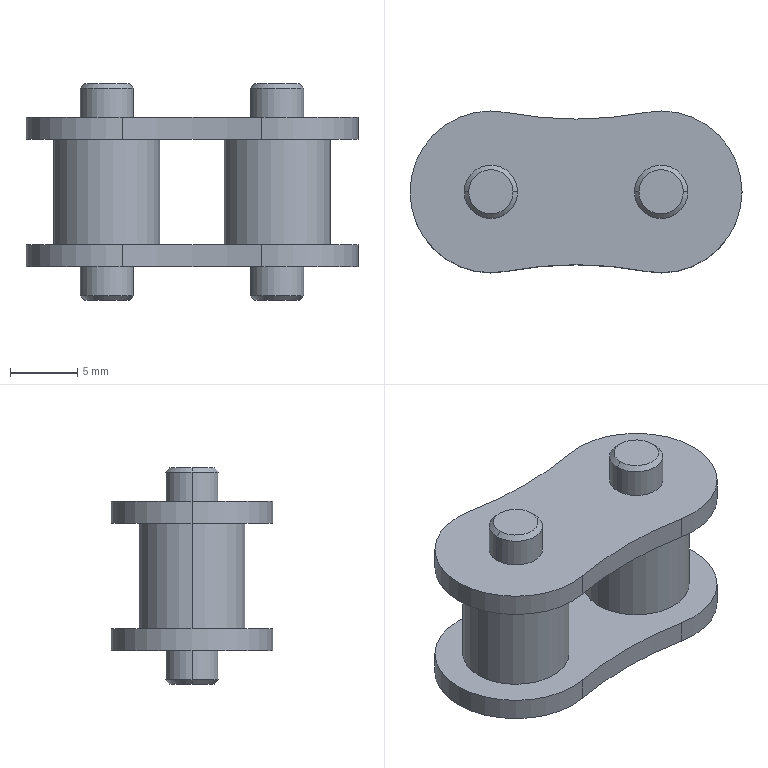Part | SolidWorks | features Boss 2, Chamfer 1, Extrusion 1, MirrorPattern 1 | 1 solid | 38 faces | box 24.77 x 12.07 x 16.175 mm | volume 1756 mm3 | cylinder 22 | cone 8 | plane 8 | commonest cylinder face diameters 3.98 x8 12.07 x6 7.92 x4 55.348 x4
STEP:
#1=CARTESIAN_POINT('',(-8.007,0.,-8.087));
#2=VERTEX_POINT('',#1);
#3=CARTESIAN_POINT('',(-4.693,0.,-8.087));
#4=VERTEX_POINT('',#3);
#5=CARTESIAN_POINT('',(-6.35,0.,-8.087));
#6=DIRECTION('',(0.,0.,-1.));
#7=DIRECTION('',(-1.,0.,0.));
#8=AXIS2_PLACEMENT_3D('',#5,#6,#7);
#9=CIRCLE('',#8,1.657);
#10=EDGE_CURVE('',#2,#4,#9,.T.);
#11=ORIENTED_EDGE('',*,*,#10,.F.);
#12=CARTESIAN_POINT('',(-8.34,0.,-7.754));
#13=VERTEX_POINT('',#12);
#14=CARTESIAN_POINT('',(-8.34,0.,-7.754));
#15=DIRECTION('',(-0.7071,0.,0.7071));
#16=VECTOR('',#15,1000.);
#17=LINE('',#14,#16);
#18=EDGE_CURVE('',#2,#13,#17,.T.);
#19=ORIENTED_EDGE('',*,*,#18,.T.);
#20=CARTESIAN_POINT('',(-4.36,0.,-7.754));
#21=VERTEX_POINT('',#20);
#22=CARTESIAN_POINT('',(-6.35,0.,-7.754));
#23=DIRECTION('',(0.,0.,1.));
#24=DIRECTION('',(-1.,0.,0.));
#25=AXIS2_PLACEMENT_3D('',#22,#23,#24);
#26=CIRCLE('',#25,1.99);
#27=EDGE_CURVE('',#21,#13,#26,.T.);
#28=ORIENTED_EDGE('',*,*,#27,.F.);
#29=CARTESIAN_POINT('',(-4.36,0.,-7.754));
#30=DIRECTION('',(0.7071,0.,0.7071));
#31=VECTOR('',#30,1000.);
#32=LINE('',#29,#31);
#33=EDGE_CURVE('',#4,#21,#32,.T.);
#34=ORIENTED_EDGE('',*,*,#33,.F.);
#35=EDGE_LOOP('',(#11,#19,#28,#34));
#36=FACE_OUTER_BOUND('',#35,.T.);
#37=CARTESIAN_POINT('',(-6.35,0.,-7.754));
#38=DIRECTION('',(0.,0.,1.));
#39=DIRECTION('',(1.,0.,0.));
#40=AXIS2_PLACEMENT_3D('',#37,#38,#39);
#41=CONICAL_SURFACE('',#40,1.99,0.7854);
#42=ADVANCED_FACE('',(#36),#41,.T.);
#43=CARTESIAN_POINT('',(4.693,0.,-8.087));
#44=VERTEX_POINT('',#43);
#45=CARTESIAN_POINT('',(8.007,0.,-8.087));
#46=VERTEX_POINT('',#45);
#47=CARTESIAN_POINT('',(6.35,0.,-8.087));
#48=DIRECTION('',(0.,0.,-1.));
#49=DIRECTION('',(-1.,0.,0.));
#50=AXIS2_PLACEMENT_3D('',#47,#48,#49);
#51=CIRCLE('',#50,1.657);
#52=EDGE_CURVE('',#44,#46,#51,.T.);
#53=ORIENTED_EDGE('',*,*,#52,.F.);
#54=CARTESIAN_POINT('',(4.36,0.,-7.754));
#55=VERTEX_POINT('',#54);
#56=CARTESIAN_POINT('',(4.36,0.,-7.754));
#57=DIRECTION('',(-0.7071,0.,0.7071));
#58=VECTOR('',#57,1000.);
#59=LINE('',#56,#58);
#60=EDGE_CURVE('',#44,#55,#59,.T.);
#61=ORIENTED_EDGE('',*,*,#60,.T.);
#62=CARTESIAN_POINT('',(8.34,0.,-7.754));
#63=VERTEX_POINT('',#62);
#64=CARTESIAN_POINT('',(6.35,0.,-7.754));
#65=DIRECTION('',(0.,0.,1.));
#66=DIRECTION('',(-1.,0.,0.));
#67=AXIS2_PLACEMENT_3D('',#64,#65,#66);
#68=CIRCLE('',#67,1.99);
#69=EDGE_CURVE('',#63,#55,#68,.T.);
#70=ORIENTED_EDGE('',*,*,#69,.F.);
#71=CARTESIAN_POINT('',(8.34,0.,-7.754));
#72=DIRECTION('',(0.7071,0.,0.7071));
#73=VECTOR('',#72,1000.);
#74=LINE('',#71,#73);
#75=EDGE_CURVE('',#46,#63,#74,.T.);
#76=ORIENTED_EDGE('',*,*,#75,.F.);
#77=EDGE_LOOP('',(#53,#61,#70,#76));
#78=FACE_OUTER_BOUND('',#77,.T.);
#79=CARTESIAN_POINT('',(6.35,0.,-7.754));
#80=DIRECTION('',(0.,0.,1.));
#81=DIRECTION('',(1.,0.,0.));
#82=AXIS2_PLACEMENT_3D('',#79,#80,#81);
#83=CONICAL_SURFACE('',#82,1.99,0.7854);
#84=ADVANCED_FACE('',(#78),#83,.T.);
#85=ORIENTED_EDGE('',*,*,#27,.T.);
#86=CARTESIAN_POINT('',(-8.34,0.,-5.59));
#87=VERTEX_POINT('',#86);
#88=CARTESIAN_POINT('',(-8.34,0.,-8.087));
#89=DIRECTION('',(0.,0.,1.));
#90=VECTOR('',#89,1000.);
#91=LINE('',#88,#90);
#92=EDGE_CURVE('',#13,#87,#91,.T.);
#93=ORIENTED_EDGE('',*,*,#92,.T.);
#94=CARTESIAN_POINT('',(-4.36,0.,-5.59));
#95=VERTEX_POINT('',#94);
#96=CARTESIAN_POINT('',(-6.35,0.,-5.59));
#97=DIRECTION('',(0.,0.,-1.));
#98=DIRECTION('',(-1.,0.,0.));
#99=AXIS2_PLACEMENT_3D('',#96,#97,#98);
#100=CIRCLE('',#99,1.99);
#101=EDGE_CURVE('',#87,#95,#100,.T.);
#102=ORIENTED_EDGE('',*,*,#101,.T.);
#103=CARTESIAN_POINT('',(-4.36,0.,-8.087));
#104=DIRECTION('',(0.,0.,1.));
#105=VECTOR('',#104,1000.);
#106=LINE('',#103,#105);
#107=EDGE_CURVE('',#21,#95,#106,.T.);
#108=ORIENTED_EDGE('',*,*,#107,.F.);
#109=EDGE_LOOP('',(#85,#93,#102,#108));
#110=FACE_OUTER_BOUND('',#109,.T.);
#111=CARTESIAN_POINT('',(-6.35,0.,-8.087));
#112=DIRECTION('',(0.,0.,1.));
#113=DIRECTION('',(1.,0.,0.));
#114=AXIS2_PLACEMENT_3D('',#111,#112,#113);
#115=CYLINDRICAL_SURFACE('',#114,1.99);
#116=ADVANCED_FACE('',(#110),#115,.T.);
#117=ORIENTED_EDGE('',*,*,#69,.T.);
#118=CARTESIAN_POINT('',(4.36,0.,-5.59));
#119=VERTEX_POINT('',#118);
#120=CARTESIAN_POINT('',(4.36,0.,-8.087));
#121=DIRECTION('',(0.,0.,1.));
#122=VECTOR('',#121,1000.);
#123=LINE('',#120,#122);
#124=EDGE_CURVE('',#55,#119,#123,.T.);
#125=ORIENTED_EDGE('',*,*,#124,.T.);
#126=CARTESIAN_POINT('',(8.34,0.,-5.59));
#127=VERTEX_POINT('',#126);
#128=CARTESIAN_POINT('',(6.35,0.,-5.59));
#129=DIRECTION('',(0.,0.,-1.));
#130=DIRECTION('',(-1.,0.,0.));
#131=AXIS2_PLACEMENT_3D('',#128,#129,#130);
#132=CIRCLE('',#131,1.99);
#133=EDGE_CURVE('',#119,#127,#132,.T.);
#134=ORIENTED_EDGE('',*,*,#133,.T.);
#135=CARTESIAN_POINT('',(8.34,0.,-8.087));
#136=DIRECTION('',(0.,0.,1.));
#137=VECTOR('',#136,1000.);
#138=LINE('',#135,#137);
#139=EDGE_CURVE('',#63,#127,#138,.T.);
#140=ORIENTED_EDGE('',*,*,#139,.F.);
#141=EDGE_LOOP('',(#117,#125,#134,#140));
#142=FACE_OUTER_BOUND('',#141,.T.);
#143=CARTESIAN_POINT('',(6.35,0.,-8.087));
#144=DIRECTION('',(0.,0.,1.));
#145=DIRECTION('',(1.,0.,0.));
#146=AXIS2_PLACEMENT_3D('',#143,#144,#145);
#147=CYLINDRICAL_SURFACE('',#146,1.99);
#148=ADVANCED_FACE('',(#142),#147,.T.);
#149=CARTESIAN_POINT('',(5.213,-5.927,-5.59));
#150=VERTEX_POINT('',#149);
#151=CARTESIAN_POINT('',(12.385,0.,-5.59));
#152=VERTEX_POINT('',#151);
#153=CARTESIAN_POINT('',(6.35,0.,-5.59));
#154=DIRECTION('',(0.,0.,1.));
#155=DIRECTION('',(1.,0.,0.));
#156=AXIS2_PLACEMENT_3D('',#153,#154,#155);
#157=CIRCLE('',#156,6.035);
#158=EDGE_CURVE('',#150,#152,#157,.T.);
#159=ORIENTED_EDGE('',*,*,#158,.T.);
#160=CARTESIAN_POINT('',(12.385,0.,-3.925));
#161=VERTEX_POINT('',#160);
#162=CARTESIAN_POINT('',(12.385,0.,-5.59));
#163=DIRECTION('',(0.,0.,1.));
#164=VECTOR('',#163,1000.);
#165=LINE('',#162,#164);
#166=EDGE_CURVE('',#152,#161,#165,.T.);
#167=ORIENTED_EDGE('',*,*,#166,.T.);
#168=CARTESIAN_POINT('',(5.213,-5.927,-3.925));
#169=VERTEX_POINT('',#168);
#170=CARTESIAN_POINT('',(6.35,0.,-3.925));
#171=DIRECTION('',(0.,0.,1.));
#172=DIRECTION('',(1.,0.,0.));
#173=AXIS2_PLACEMENT_3D('',#170,#171,#172);
#174=CIRCLE('',#173,6.035);
#175=EDGE_CURVE('',#169,#161,#174,.T.);
#176=ORIENTED_EDGE('',*,*,#175,.F.);
#177=CARTESIAN_POINT('',(5.213,-5.927,-5.59));
#178=DIRECTION('',(0.,0.,1.));
#179=VECTOR('',#178,1000.);
#180=LINE('',#177,#179);
#181=EDGE_CURVE('',#150,#169,#180,.T.);
#182=ORIENTED_EDGE('',*,*,#181,.F.);
#183=EDGE_LOOP('',(#159,#167,#176,#182));
#184=FACE_OUTER_BOUND('',#183,.T.);
#185=CARTESIAN_POINT('',(6.35,0.,-5.59));
#186=DIRECTION('',(0.,0.,1.));
#187=DIRECTION('',(1.,0.,0.));
#188=AXIS2_PLACEMENT_3D('',#185,#186,#187);
#189=CYLINDRICAL_SURFACE('',#188,6.035);
#190=ADVANCED_FACE('',(#184),#189,.T.);
#191=CARTESIAN_POINT('',(-4.693,0.,8.087));
#192=VERTEX_POINT('',#191);
#193=CARTESIAN_POINT('',(-8.007,0.,8.087));
#194=VERTEX_POINT('',#193);
#195=CARTESIAN_POINT('',(-6.35,0.,8.087));
#196=DIRECTION('',(0.,0.,1.));
#197=DIRECTION('',(1.,0.,0.));
#198=AXIS2_PLACEMENT_3D('',#195,#196,#197);
#199=CIRCLE('',#198,1.657);
#200=EDGE_CURVE('',#192,#194,#199,.T.);
#201=ORIENTED_EDGE('',*,*,#200,.F.);
#202=CARTESIAN_POINT('',(-4.36,0.,7.754));
#203=VERTEX_POINT('',#202);
#204=CARTESIAN_POINT('',(-4.693,0.,8.087));
#205=DIRECTION('',(0.7071,0.,-0.7071));
#206=VECTOR('',#205,1000.);
#207=LINE('',#204,#206);
#208=EDGE_CURVE('',#192,#203,#207,.T.);
#209=ORIENTED_EDGE('',*,*,#208,.T.);
#210=CARTESIAN_POINT('',(-8.34,0.,7.754));
#211=VERTEX_POINT('',#210);
#212=CARTESIAN_POINT('',(-6.35,0.,7.754));
#213=DIRECTION('',(0.,0.,-1.));
#214=DIRECTION('',(1.,0.,0.));
#215=AXIS2_PLACEMENT_3D('',#212,#213,#214);
#216=CIRCLE('',#215,1.99);
#217=EDGE_CURVE('',#211,#203,#216,.T.);
#218=ORIENTED_EDGE('',*,*,#217,.F.);
#219=CARTESIAN_POINT('',(-8.007,0.,8.087));
#220=DIRECTION('',(-0.7071,0.,-0.7071));
#221=VECTOR('',#220,1000.);
#222=LINE('',#219,#221);
#223=EDGE_CURVE('',#194,#211,#222,.T.);
#224=ORIENTED_EDGE('',*,*,#223,.F.);
#225=EDGE_LOOP('',(#201,#209,#218,#224));
#226=FACE_OUTER_BOUND('',#225,.T.);
#227=CARTESIAN_POINT('',(-6.35,0.,8.087));
#228=DIRECTION('',(0.,0.,-1.));
#229=DIRECTION('',(-1.,0.,0.));
#230=AXIS2_PLACEMENT_3D('',#227,#228,#229);
#231=CONICAL_SURFACE('',#230,1.657,0.7854);
#232=ADVANCED_FACE('',(#226),#231,.T.);
#233=CARTESIAN_POINT('',(8.007,0.,8.087));
#234=VERTEX_POINT('',#233);
#235=CARTESIAN_POINT('',(4.693,0.,8.087));
#236=VERTEX_POINT('',#235);
#237=CARTESIAN_POINT('',(6.35,0.,8.087));
#238=DIRECTION('',(0.,0.,1.));
#239=DIRECTION('',(1.,0.,0.));
#240=AXIS2_PLACEMENT_3D('',#237,#238,#239);
#241=CIRCLE('',#240,1.657);
#242=EDGE_CURVE('',#234,#236,#241,.T.);
#243=ORIENTED_EDGE('',*,*,#242,.F.);
#244=CARTESIAN_POINT('',(8.34,0.,7.754));
#245=VERTEX_POINT('',#244);
#246=CARTESIAN_POINT('',(8.007,0.,8.087));
#247=DIRECTION('',(0.7071,0.,-0.7071));
#248=VECTOR('',#247,1000.);
#249=LINE('',#246,#248);
#250=EDGE_CURVE('',#234,#245,#249,.T.);
#251=ORIENTED_EDGE('',*,*,#250,.T.);
#252=CARTESIAN_POINT('',(4.36,0.,7.754));
#253=VERTEX_POINT('',#252);
#254=CARTESIAN_POINT('',(6.35,0.,7.754));
#255=DIRECTION('',(0.,0.,-1.));
#256=DIRECTION('',(1.,0.,0.));
#257=AXIS2_PLACEMENT_3D('',#254,#255,#256);
#258=CIRCLE('',#257,1.99);
#259=EDGE_CURVE('',#253,#245,#258,.T.);
#260=ORIENTED_EDGE('',*,*,#259,.F.);
#261=CARTESIAN_POINT('',(4.693,0.,8.087));
#262=DIRECTION('',(-0.7071,0.,-0.7071));
#263=VECTOR('',#262,1000.);
#264=LINE('',#261,#263);
#265=EDGE_CURVE('',#236,#253,#264,.T.);
#266=ORIENTED_EDGE('',*,*,#265,.F.);
#267=EDGE_LOOP('',(#243,#251,#260,#266));
#268=FACE_OUTER_BOUND('',#267,.T.);
#269=CARTESIAN_POINT('',(6.35,0.,8.087));
#270=DIRECTION('',(0.,0.,-1.));
#271=DIRECTION('',(-1.,0.,0.));
#272=AXIS2_PLACEMENT_3D('',#269,#270,#271);
#273=CONICAL_SURFACE('',#272,1.657,0.7854);
#274=ADVANCED_FACE('',(#268),#273,.T.);
#275=ORIENTED_EDGE('',*,*,#217,.T.);
#276=CARTESIAN_POINT('',(-4.36,0.,5.59));
#277=VERTEX_POINT('',#276);
#278=CARTESIAN_POINT('',(-4.36,0.,8.087));
#279=DIRECTION('',(0.,0.,-1.));
#280=VECTOR('',#279,1000.);
#281=LINE('',#278,#280);
#282=EDGE_CURVE('',#203,#277,#281,.T.);
#283=ORIENTED_EDGE('',*,*,#282,.T.);
#284=CARTESIAN_POINT('',(-8.34,0.,5.59));
#285=VERTEX_POINT('',#284);
#286=CARTESIAN_POINT('',(-6.35,0.,5.59));
#287=DIRECTION('',(0.,0.,1.));
#288=DIRECTION('',(1.,0.,0.));
#289=AXIS2_PLACEMENT_3D('',#286,#287,#288);
#290=CIRCLE('',#289,1.99);
#291=EDGE_CURVE('',#277,#285,#290,.T.);
#292=ORIENTED_EDGE('',*,*,#291,.T.);
#293=CARTESIAN_POINT('',(-8.34,0.,8.087));
#294=DIRECTION('',(0.,0.,-1.));
#295=VECTOR('',#294,1000.);
#296=LINE('',#293,#295);
#297=EDGE_CURVE('',#211,#285,#296,.T.);
#298=ORIENTED_EDGE('',*,*,#297,.F.);
#299=EDGE_LOOP('',(#275,#283,#292,#298));
#300=FACE_OUTER_BOUND('',#299,.T.);
#301=CARTESIAN_POINT('',(-6.35,0.,8.087));
#302=DIRECTION('',(0.,0.,-1.));
#303=DIRECTION('',(-1.,0.,0.));
#304=AXIS2_PLACEMENT_3D('',#301,#302,#303);
#305=CYLINDRICAL_SURFACE('',#304,1.99);
#306=ADVANCED_FACE('',(#300),#305,.T.);
#307=ORIENTED_EDGE('',*,*,#259,.T.);
#308=CARTESIAN_POINT('',(8.34,0.,5.59));
#309=VERTEX_POINT('',#308);
#310=CARTESIAN_POINT('',(8.34,0.,8.087));
#311=DIRECTION('',(0.,0.,-1.));
#312=VECTOR('',#311,1000.);
#313=LINE('',#310,#312);
#314=EDGE_CURVE('',#245,#309,#313,.T.);
#315=ORIENTED_EDGE('',*,*,#314,.T.);
#316=CARTESIAN_POINT('',(4.36,0.,5.59));
#317=VERTEX_POINT('',#316);
#318=CARTESIAN_POINT('',(6.35,0.,5.59));
#319=DIRECTION('',(0.,0.,1.));
#320=DIRECTION('',(1.,0.,0.));
#321=AXIS2_PLACEMENT_3D('',#318,#319,#320);
#322=CIRCLE('',#321,1.99);
#323=EDGE_CURVE('',#309,#317,#322,.T.);
#324=ORIENTED_EDGE('',*,*,#323,.T.);
#325=CARTESIAN_POINT('',(4.36,0.,8.087));
#326=DIRECTION('',(0.,0.,-1.));
#327=VECTOR('',#326,1000.);
#328=LINE('',#325,#327);
#329=EDGE_CURVE('',#253,#317,#328,.T.);
#330=ORIENTED_EDGE('',*,*,#329,.F.);
#331=EDGE_LOOP('',(#307,#315,#324,#330));
#332=FACE_OUTER_BOUND('',#331,.T.);
#333=CARTESIAN_POINT('',(6.35,0.,8.087));
#334=DIRECTION('',(0.,0.,-1.));
#335=DIRECTION('',(-1.,0.,0.));
#336=AXIS2_PLACEMENT_3D('',#333,#334,#335);
#337=CYLINDRICAL_SURFACE('',#336,1.99);
#338=ADVANCED_FACE('',(#332),#337,.T.);
#339=CARTESIAN_POINT('',(-10.31,0.,3.925));
#340=VERTEX_POINT('',#339);
#341=CARTESIAN_POINT('',(-2.39,0.,3.925));
#342=VERTEX_POINT('',#341);
#343=CARTESIAN_POINT('',(-6.35,0.,3.925));
#344=DIRECTION('',(0.,0.,-1.));
#345=DIRECTION('',(1.,0.,0.));
#346=AXIS2_PLACEMENT_3D('',#343,#344,#345);
#347=CIRCLE('',#346,3.96);
#348=EDGE_CURVE('',#340,#342,#347,.T.);
#349=ORIENTED_EDGE('',*,*,#348,.T.);
#350=CARTESIAN_POINT('',(-2.39,0.,-3.925));
#351=VERTEX_POINT('',#350);
#352=CARTESIAN_POINT('',(-2.39,0.,3.925));
#353=DIRECTION('',(0.,0.,-1.));
#354=VECTOR('',#353,1000.);
#355=LINE('',#352,#354);
#356=EDGE_CURVE('',#342,#351,#355,.T.);
#357=ORIENTED_EDGE('',*,*,#356,.T.);
#358=CARTESIAN_POINT('',(-10.31,0.,-3.925));
#359=VERTEX_POINT('',#358);
#360=CARTESIAN_POINT('',(-6.35,0.,-3.925));
#361=DIRECTION('',(0.,0.,-1.));
#362=DIRECTION('',(-1.,0.,0.));
#363=AXIS2_PLACEMENT_3D('',#360,#361,#362);
#364=CIRCLE('',#363,3.96);
#365=EDGE_CURVE('',#359,#351,#364,.T.);
#366=ORIENTED_EDGE('',*,*,#365,.F.);
#367=CARTESIAN_POINT('',(-10.31,0.,3.925));
#368=DIRECTION('',(0.,0.,-1.));
#369=VECTOR('',#368,1000.);
#370=LINE('',#367,#369);
#371=EDGE_CURVE('',#340,#359,#370,.T.);
#372=ORIENTED_EDGE('',*,*,#371,.F.);
#373=EDGE_LOOP('',(#349,#357,#366,#372));
#374=FACE_OUTER_BOUND('',#373,.T.);
#375=CARTESIAN_POINT('',(-6.35,0.,3.925));
#376=DIRECTION('',(0.,0.,-1.));
#377=DIRECTION('',(-1.,0.,0.));
#378=AXIS2_PLACEMENT_3D('',#375,#376,#377);
#379=CYLINDRICAL_SURFACE('',#378,3.96);
#380=ADVANCED_FACE('',(#374),#379,.T.);
#381=CARTESIAN_POINT('',(-12.385,0.,5.59));
#382=VERTEX_POINT('',#381);
#383=CARTESIAN_POINT('',(-5.213,-5.927,5.59));
#384=VERTEX_POINT('',#383);
#385=CARTESIAN_POINT('',(-6.35,0.,5.59));
#386=DIRECTION('',(0.,0.,1.));
#387=DIRECTION('',(1.,0.,0.));
#388=AXIS2_PLACEMENT_3D('',#385,#386,#387);
#389=CIRCLE('',#388,6.035);
#390=EDGE_CURVE('',#382,#384,#389,.T.);
#391=ORIENTED_EDGE('',*,*,#390,.F.);
#392=CARTESIAN_POINT('',(-12.385,0.,3.925));
#393=VERTEX_POINT('',#392);
#394=CARTESIAN_POINT('',(-12.385,0.,5.59));
#395=DIRECTION('',(0.,0.,-1.));
#396=VECTOR('',#395,1000.);
#397=LINE('',#394,#396);
#398=EDGE_CURVE('',#382,#393,#397,.T.);
#399=ORIENTED_EDGE('',*,*,#398,.T.);
#400=CARTESIAN_POINT('',(-5.213,-5.927,3.925));
#401=VERTEX_POINT('',#400);
#402=CARTESIAN_POINT('',(-6.35,0.,3.925));
#403=DIRECTION('',(0.,0.,1.));
#404=DIRECTION('',(1.,0.,0.));
#405=AXIS2_PLACEMENT_3D('',#402,#403,#404);
#406=CIRCLE('',#405,6.035);
#407=EDGE_CURVE('',#393,#401,#406,.T.);
#408=ORIENTED_EDGE('',*,*,#407,.T.);
#409=CARTESIAN_POINT('',(-5.213,-5.927,5.59));
#410=DIRECTION('',(0.,0.,-1.));
#411=VECTOR('',#410,1000.);
#412=LINE('',#409,#411);
#413=EDGE_CURVE('',#384,#401,#412,.T.);
#414=ORIENTED_EDGE('',*,*,#413,.F.);
#415=EDGE_LOOP('',(#391,#399,#408,#414));
#416=FACE_OUTER_BOUND('',#415,.T.);
#417=CARTESIAN_POINT('',(-6.35,0.,5.59));
#418=DIRECTION('',(0.,0.,-1.));
#419=DIRECTION('',(-1.,0.,0.));
#420=AXIS2_PLACEMENT_3D('',#417,#418,#419);
#421=CYLINDRICAL_SURFACE('',#420,6.035);
#422=ADVANCED_FACE('',(#416),#421,.T.);
#423=CARTESIAN_POINT('',(10.31,0.,3.925));
#424=VERTEX_POINT('',#423);
#425=CARTESIAN_POINT('',(2.39,0.,3.925));
#426=VERTEX_POINT('',#425);
#427=CARTESIAN_POINT('',(6.35,0.,3.925));
#428=DIRECTION('',(0.,0.,1.));
#429=DIRECTION('',(1.,0.,0.));
#430=AXIS2_PLACEMENT_3D('',#427,#428,#429);
#431=CIRCLE('',#430,3.96);
#432=EDGE_CURVE('',#424,#426,#431,.T.);
#433=ORIENTED_EDGE('',*,*,#432,.F.);
#434=CARTESIAN_POINT('',(10.31,0.,-3.925));
#435=VERTEX_POINT('',#434);
#436=CARTESIAN_POINT('',(10.31,0.,3.925));
#437=DIRECTION('',(0.,0.,-1.));
#438=VECTOR('',#437,1000.);
#439=LINE('',#436,#438);
#440=EDGE_CURVE('',#424,#435,#439,.T.);
#441=ORIENTED_EDGE('',*,*,#440,.T.);
#442=CARTESIAN_POINT('',(2.39,0.,-3.925));
#443=VERTEX_POINT('',#442);
#444=CARTESIAN_POINT('',(6.35,0.,-3.925));
#445=DIRECTION('',(0.,0.,-1.));
#446=DIRECTION('',(-1.,0.,0.));
#447=AXIS2_PLACEMENT_3D('',#444,#445,#446);
#448=CIRCLE('',#447,3.96);
#449=EDGE_CURVE('',#443,#435,#448,.T.);
#450=ORIENTED_EDGE('',*,*,#449,.F.);
#451=CARTESIAN_POINT('',(2.39,0.,3.925));
#452=DIRECTION('',(0.,0.,-1.));
#453=VECTOR('',#452,1000.);
#454=LINE('',#451,#453);
#455=EDGE_CURVE('',#426,#443,#454,.T.);
#456=ORIENTED_EDGE('',*,*,#455,.F.);
#457=EDGE_LOOP('',(#433,#441,#450,#456));
#458=FACE_OUTER_BOUND('',#457,.T.);
#459=CARTESIAN_POINT('',(6.35,0.,3.925));
#460=DIRECTION('',(0.,0.,-1.));
#461=DIRECTION('',(-1.,0.,0.));
#462=AXIS2_PLACEMENT_3D('',#459,#460,#461);
#463=CYLINDRICAL_SURFACE('',#462,3.96);
#464=ADVANCED_FACE('',(#458),#463,.T.);
#465=CARTESIAN_POINT('',(6.35,0.,5.59));
#466=DIRECTION('',(0.,0.,1.));
#467=DIRECTION('',(1.,0.,0.));
#468=AXIS2_PLACEMENT_3D('',#465,#466,#467);
#469=CIRCLE('',#468,1.99);
#470=EDGE_CURVE('',#317,#309,#469,.T.);
#471=ORIENTED_EDGE('',*,*,#470,.F.);
#472=ORIENTED_EDGE('',*,*,#323,.F.);
#473=EDGE_LOOP('',(#471,#472));
#474=FACE_BOUND('',#473,.T.);
#475=CARTESIAN_POINT('',(5.213,-5.927,5.59));
#476=VERTEX_POINT('',#475);
#477=CARTESIAN_POINT('',(0.,-33.105,5.59));
#478=DIRECTION('',(0.,0.,-1.));
#479=DIRECTION('',(1.,0.,0.));
#480=AXIS2_PLACEMENT_3D('',#477,#478,#479);
#481=CIRCLE('',#480,27.674);
#482=EDGE_CURVE('',#384,#476,#481,.T.);
#483=ORIENTED_EDGE('',*,*,#482,.T.);
#484=CARTESIAN_POINT('',(5.213,5.927,5.59));
#485=VERTEX_POINT('',#484);
#486=CARTESIAN_POINT('',(6.35,0.,5.59));
#487=DIRECTION('',(0.,0.,1.));
#488=DIRECTION('',(1.,0.,0.));
#489=AXIS2_PLACEMENT_3D('',#486,#487,#488);
#490=CIRCLE('',#489,6.035);
#491=EDGE_CURVE('',#476,#485,#490,.T.);
#492=ORIENTED_EDGE('',*,*,#491,.T.);
#493=CARTESIAN_POINT('',(-5.213,5.927,5.59));
#494=VERTEX_POINT('',#493);
#495=CARTESIAN_POINT('',(0.,33.105,5.59));
#496=DIRECTION('',(0.,0.,-1.));
#497=DIRECTION('',(1.,0.,0.));
#498=AXIS2_PLACEMENT_3D('',#495,#496,#497);
#499=CIRCLE('',#498,27.674);
#500=EDGE_CURVE('',#485,#494,#499,.T.);
#501=ORIENTED_EDGE('',*,*,#500,.T.);
#502=CARTESIAN_POINT('',(-6.35,0.,5.59));
#503=DIRECTION('',(0.,0.,1.));
#504=DIRECTION('',(1.,0.,0.));
#505=AXIS2_PLACEMENT_3D('',#502,#503,#504);
#506=CIRCLE('',#505,6.035);
#507=EDGE_CURVE('',#494,#382,#506,.T.);
#508=ORIENTED_EDGE('',*,*,#507,.T.);
#509=ORIENTED_EDGE('',*,*,#390,.T.);
#510=EDGE_LOOP('',(#483,#492,#501,#508,#509));
#511=FACE_OUTER_BOUND('',#510,.T.);
#512=CARTESIAN_POINT('',(-6.35,0.,5.59));
#513=DIRECTION('',(0.,0.,1.));
#514=DIRECTION('',(1.,0.,0.));
#515=AXIS2_PLACEMENT_3D('',#512,#513,#514);
#516=CIRCLE('',#515,1.99);
#517=EDGE_CURVE('',#285,#277,#516,.T.);
#518=ORIENTED_EDGE('',*,*,#517,.F.);
#519=ORIENTED_EDGE('',*,*,#291,.F.);
#520=EDGE_LOOP('',(#518,#519));
#521=FACE_BOUND('',#520,.T.);
#522=CARTESIAN_POINT('',(-3.175,-16.553,5.59));
#523=DIRECTION('',(0.,0.,1.));
#524=DIRECTION('',(1.,0.,0.));
#525=AXIS2_PLACEMENT_3D('',#522,#523,#524);
#526=PLANE('',#525);
#527=ADVANCED_FACE('',(#474,#511,#521),#526,.T.);
#528=CARTESIAN_POINT('',(5.213,-5.927,3.925));
#529=VERTEX_POINT('',#528);
#530=CARTESIAN_POINT('',(0.,-33.105,3.925));
#531=DIRECTION('',(0.,0.,-1.));
#532=DIRECTION('',(1.,0.,0.));
#533=AXIS2_PLACEMENT_3D('',#530,#531,#532);
#534=CIRCLE('',#533,27.674);
#535=EDGE_CURVE('',#401,#529,#534,.T.);
#536=ORIENTED_EDGE('',*,*,#535,.F.);
#537=ORIENTED_EDGE('',*,*,#407,.F.);
#538=CARTESIAN_POINT('',(-5.213,5.927,3.925));
#539=VERTEX_POINT('',#538);
#540=CARTESIAN_POINT('',(-6.35,0.,3.925));
#541=DIRECTION('',(0.,0.,1.));
#542=DIRECTION('',(1.,0.,0.));
#543=AXIS2_PLACEMENT_3D('',#540,#541,#542);
#544=CIRCLE('',#543,6.035);
#545=EDGE_CURVE('',#539,#393,#544,.T.);
#546=ORIENTED_EDGE('',*,*,#545,.F.);
#547=CARTESIAN_POINT('',(5.213,5.927,3.925));
#548=VERTEX_POINT('',#547);
#549=CARTESIAN_POINT('',(0.,33.105,3.925));
#550=DIRECTION('',(0.,0.,-1.));
#551=DIRECTION('',(1.,0.,0.));
#552=AXIS2_PLACEMENT_3D('',#549,#550,#551);
#553=CIRCLE('',#552,27.674);
#554=EDGE_CURVE('',#548,#539,#553,.T.);
#555=ORIENTED_EDGE('',*,*,#554,.F.);
#556=CARTESIAN_POINT('',(6.35,0.,3.925));
#557=DIRECTION('',(0.,0.,1.));
#558=DIRECTION('',(1.,0.,0.));
#559=AXIS2_PLACEMENT_3D('',#556,#557,#558);
#560=CIRCLE('',#559,6.035);
#561=EDGE_CURVE('',#529,#548,#560,.T.);
#562=ORIENTED_EDGE('',*,*,#561,.F.);
#563=EDGE_LOOP('',(#536,#537,#546,#555,#562));
#564=FACE_OUTER_BOUND('',#563,.T.);
#565=CARTESIAN_POINT('',(6.35,0.,3.925));
#566=DIRECTION('',(0.,0.,1.));
#567=DIRECTION('',(1.,0.,0.));
#568=AXIS2_PLACEMENT_3D('',#565,#566,#567);
#569=CIRCLE('',#568,3.96);
#570=EDGE_CURVE('',#426,#424,#569,.T.);
#571=ORIENTED_EDGE('',*,*,#570,.T.);
#572=ORIENTED_EDGE('',*,*,#432,.T.);
#573=EDGE_LOOP('',(#571,#572));
#574=FACE_BOUND('',#573,.T.);
#575=ORIENTED_EDGE('',*,*,#348,.F.);
#576=CARTESIAN_POINT('',(-6.35,0.,3.925));
#577=DIRECTION('',(0.,0.,-1.));
#578=DIRECTION('',(1.,0.,0.));
#579=AXIS2_PLACEMENT_3D('',#576,#577,#578);
#580=CIRCLE('',#579,3.96);
#581=EDGE_CURVE('',#342,#340,#580,.T.);
#582=ORIENTED_EDGE('',*,*,#581,.F.);
#583=EDGE_LOOP('',(#575,#582));
#584=FACE_BOUND('',#583,.T.);
#585=CARTESIAN_POINT('',(-3.175,-16.553,3.925));
#586=DIRECTION('',(0.,0.,1.));
#587=DIRECTION('',(1.,0.,0.));
#588=AXIS2_PLACEMENT_3D('',#585,#586,#587);
#589=PLANE('',#588);
#590=ADVANCED_FACE('',(#564,#574,#584),#589,.F.);
#591=ORIENTED_EDGE('',*,*,#440,.F.);
#592=ORIENTED_EDGE('',*,*,#570,.F.);
#593=ORIENTED_EDGE('',*,*,#455,.T.);
#594=CARTESIAN_POINT('',(6.35,0.,-3.925));
#595=DIRECTION('',(0.,0.,-1.));
#596=DIRECTION('',(-1.,0.,0.));
#597=AXIS2_PLACEMENT_3D('',#594,#595,#596);
#598=CIRCLE('',#597,3.96);
#599=EDGE_CURVE('',#435,#443,#598,.T.);
#600=ORIENTED_EDGE('',*,*,#599,.F.);
#601=EDGE_LOOP('',(#591,#592,#593,#600));
#602=FACE_OUTER_BOUND('',#601,.T.);
#603=CARTESIAN_POINT('',(6.35,0.,3.925));
#604=DIRECTION('',(0.,0.,-1.));
#605=DIRECTION('',(-1.,0.,0.));
#606=AXIS2_PLACEMENT_3D('',#603,#604,#605);
#607=CYLINDRICAL_SURFACE('',#606,3.96);
#608=ADVANCED_FACE('',(#602),#607,.T.);
#609=ORIENTED_EDGE('',*,*,#535,.T.);
#610=CARTESIAN_POINT('',(5.213,-5.927,5.59));
#611=DIRECTION('',(0.,0.,-1.));
#612=VECTOR('',#611,1000.);
#613=LINE('',#610,#612);
#614=EDGE_CURVE('',#476,#529,#613,.T.);
#615=ORIENTED_EDGE('',*,*,#614,.F.);
#616=ORIENTED_EDGE('',*,*,#482,.F.);
#617=ORIENTED_EDGE('',*,*,#413,.T.);
#618=EDGE_LOOP('',(#609,#615,#616,#617));
#619=FACE_OUTER_BOUND('',#618,.T.);
#620=CARTESIAN_POINT('',(0.,-33.105,5.59));
#621=DIRECTION('',(0.,0.,-1.));
#622=DIRECTION('',(-1.,0.,0.));
#623=AXIS2_PLACEMENT_3D('',#620,#621,#622);
#624=CYLINDRICAL_SURFACE('',#623,27.674);
#625=ADVANCED_FACE('',(#619),#624,.F.);
#626=ORIENTED_EDGE('',*,*,#561,.T.);
#627=CARTESIAN_POINT('',(5.213,5.927,5.59));
#628=DIRECTION('',(0.,0.,-1.));
#629=VECTOR('',#628,1000.);
#630=LINE('',#627,#629);
#631=EDGE_CURVE('',#485,#548,#630,.T.);
#632=ORIENTED_EDGE('',*,*,#631,.F.);
#633=ORIENTED_EDGE('',*,*,#491,.F.);
#634=ORIENTED_EDGE('',*,*,#614,.T.);
#635=EDGE_LOOP('',(#626,#632,#633,#634));
#636=FACE_OUTER_BOUND('',#635,.T.);
#637=CARTESIAN_POINT('',(6.35,0.,5.59));
#638=DIRECTION('',(0.,0.,-1.));
#639=DIRECTION('',(-1.,0.,0.));
#640=AXIS2_PLACEMENT_3D('',#637,#638,#639);
#641=CYLINDRICAL_SURFACE('',#640,6.035);
#642=ADVANCED_FACE('',(#636),#641,.T.);
#643=ORIENTED_EDGE('',*,*,#554,.T.);
#644=CARTESIAN_POINT('',(-5.213,5.927,5.59));
#645=DIRECTION('',(0.,0.,-1.));
#646=VECTOR('',#645,1000.);
#647=LINE('',#644,#646);
#648=EDGE_CURVE('',#494,#539,#647,.T.);
#649=ORIENTED_EDGE('',*,*,#648,.F.);
#650=ORIENTED_EDGE('',*,*,#500,.F.);
#651=ORIENTED_EDGE('',*,*,#631,.T.);
#652=EDGE_LOOP('',(#643,#649,#650,#651));
#653=FACE_OUTER_BOUND('',#652,.T.);
#654=CARTESIAN_POINT('',(0.,33.105,5.59));
#655=DIRECTION('',(0.,0.,-1.));
#656=DIRECTION('',(-1.,0.,0.));
#657=AXIS2_PLACEMENT_3D('',#654,#655,#656);
#658=CYLINDRICAL_SURFACE('',#657,27.674);
#659=ADVANCED_FACE('',(#653),#658,.F.);
#660=ORIENTED_EDGE('',*,*,#398,.F.);
#661=ORIENTED_EDGE('',*,*,#507,.F.);
#662=ORIENTED_EDGE('',*,*,#648,.T.);
#663=ORIENTED_EDGE('',*,*,#545,.T.);
#664=EDGE_LOOP('',(#660,#661,#662,#663));
#665=FACE_OUTER_BOUND('',#664,.T.);
#666=CARTESIAN_POINT('',(-6.35,0.,5.59));
#667=DIRECTION('',(0.,0.,-1.));
#668=DIRECTION('',(-1.,0.,0.));
#669=AXIS2_PLACEMENT_3D('',#666,#667,#668);
#670=CYLINDRICAL_SURFACE('',#669,6.035);
#671=ADVANCED_FACE('',(#665),#670,.T.);
#672=ORIENTED_EDGE('',*,*,#356,.F.);
#673=ORIENTED_EDGE('',*,*,#581,.T.);
#674=ORIENTED_EDGE('',*,*,#371,.T.);
#675=CARTESIAN_POINT('',(-6.35,0.,-3.925));
#676=DIRECTION('',(0.,0.,-1.));
#677=DIRECTION('',(-1.,0.,0.));
#678=AXIS2_PLACEMENT_3D('',#675,#676,#677);
#679=CIRCLE('',#678,3.96);
#680=EDGE_CURVE('',#351,#359,#679,.T.);
#681=ORIENTED_EDGE('',*,*,#680,.F.);
#682=EDGE_LOOP('',(#672,#673,#674,#681));
#683=FACE_OUTER_BOUND('',#682,.T.);
#684=CARTESIAN_POINT('',(-6.35,0.,3.925));
#685=DIRECTION('',(0.,0.,-1.));
#686=DIRECTION('',(-1.,0.,0.));
#687=AXIS2_PLACEMENT_3D('',#684,#685,#686);
#688=CYLINDRICAL_SURFACE('',#687,3.96);
#689=ADVANCED_FACE('',(#683),#688,.T.);
#690=ORIENTED_EDGE('',*,*,#314,.F.);
#691=CARTESIAN_POINT('',(6.35,0.,7.754));
#692=DIRECTION('',(0.,0.,-1.));
#693=DIRECTION('',(1.,0.,0.));
#694=AXIS2_PLACEMENT_3D('',#691,#692,#693);
#695=CIRCLE('',#694,1.99);
#696=EDGE_CURVE('',#245,#253,#695,.T.);
#697=ORIENTED_EDGE('',*,*,#696,.T.);
#698=ORIENTED_EDGE('',*,*,#329,.T.);
#699=ORIENTED_EDGE('',*,*,#470,.T.);
#700=EDGE_LOOP('',(#690,#697,#698,#699));
#701=FACE_OUTER_BOUND('',#700,.T.);
#702=CARTESIAN_POINT('',(6.35,0.,8.087));
#703=DIRECTION('',(0.,0.,-1.));
#704=DIRECTION('',(-1.,0.,0.));
#705=AXIS2_PLACEMENT_3D('',#702,#703,#704);
#706=CYLINDRICAL_SURFACE('',#705,1.99);
#707=ADVANCED_FACE('',(#701),#706,.T.);
#708=CARTESIAN_POINT('',(6.35,0.,8.087));
#709=DIRECTION('',(0.,0.,1.));
#710=DIRECTION('',(1.,0.,0.));
#711=AXIS2_PLACEMENT_3D('',#708,#709,#710);
#712=CIRCLE('',#711,1.657);
#713=EDGE_CURVE('',#236,#234,#712,.T.);
#714=ORIENTED_EDGE('',*,*,#713,.T.);
#715=ORIENTED_EDGE('',*,*,#242,.T.);
#716=EDGE_LOOP('',(#714,#715));
#717=FACE_OUTER_BOUND('',#716,.T.);
#718=CARTESIAN_POINT('',(6.35,0.,8.087));
#719=DIRECTION('',(0.,0.,1.));
#720=DIRECTION('',(1.,0.,0.));
#721=AXIS2_PLACEMENT_3D('',#718,#719,#720);
#722=PLANE('',#721);
#723=ADVANCED_FACE('',(#717),#722,.T.);
#724=ORIENTED_EDGE('',*,*,#282,.F.);
#725=CARTESIAN_POINT('',(-6.35,0.,7.754));
#726=DIRECTION('',(0.,0.,-1.));
#727=DIRECTION('',(1.,0.,0.));
#728=AXIS2_PLACEMENT_3D('',#725,#726,#727);
#729=CIRCLE('',#728,1.99);
#730=EDGE_CURVE('',#203,#211,#729,.T.);
#731=ORIENTED_EDGE('',*,*,#730,.T.);
#732=ORIENTED_EDGE('',*,*,#297,.T.);
#733=ORIENTED_EDGE('',*,*,#517,.T.);
#734=EDGE_LOOP('',(#724,#731,#732,#733));
#735=FACE_OUTER_BOUND('',#734,.T.);
#736=CARTESIAN_POINT('',(-6.35,0.,8.087));
#737=DIRECTION('',(0.,0.,-1.));
#738=DIRECTION('',(-1.,0.,0.));
#739=AXIS2_PLACEMENT_3D('',#736,#737,#738);
#740=CYLINDRICAL_SURFACE('',#739,1.99);
#741=ADVANCED_FACE('',(#735),#740,.T.);
#742=CARTESIAN_POINT('',(-6.35,0.,8.087));
#743=DIRECTION('',(0.,0.,1.));
#744=DIRECTION('',(1.,0.,0.));
#745=AXIS2_PLACEMENT_3D('',#742,#743,#744);
#746=CIRCLE('',#745,1.657);
#747=EDGE_CURVE('',#194,#192,#746,.T.);
#748=ORIENTED_EDGE('',*,*,#747,.T.);
#749=ORIENTED_EDGE('',*,*,#200,.T.);
#750=EDGE_LOOP('',(#748,#749));
#751=FACE_OUTER_BOUND('',#750,.T.);
#752=CARTESIAN_POINT('',(-6.35,0.,8.087));
#753=DIRECTION('',(0.,0.,1.));
#754=DIRECTION('',(1.,0.,0.));
#755=AXIS2_PLACEMENT_3D('',#752,#753,#754);
#756=PLANE('',#755);
#757=ADVANCED_FACE('',(#751),#756,.T.);
#758=ORIENTED_EDGE('',*,*,#250,.F.);
#759=ORIENTED_EDGE('',*,*,#713,.F.);
#760=ORIENTED_EDGE('',*,*,#265,.T.);
#761=ORIENTED_EDGE('',*,*,#696,.F.);
#762=EDGE_LOOP('',(#758,#759,#760,#761));
#763=FACE_OUTER_BOUND('',#762,.T.);
#764=CARTESIAN_POINT('',(6.35,0.,8.087));
#765=DIRECTION('',(0.,0.,-1.));
#766=DIRECTION('',(-1.,0.,0.));
#767=AXIS2_PLACEMENT_3D('',#764,#765,#766);
#768=CONICAL_SURFACE('',#767,1.657,0.7854);
#769=ADVANCED_FACE('',(#763),#768,.T.);
#770=ORIENTED_EDGE('',*,*,#208,.F.);
#771=ORIENTED_EDGE('',*,*,#747,.F.);
#772=ORIENTED_EDGE('',*,*,#223,.T.);
#773=ORIENTED_EDGE('',*,*,#730,.F.);
#774=EDGE_LOOP('',(#770,#771,#772,#773));
#775=FACE_OUTER_BOUND('',#774,.T.);
#776=CARTESIAN_POINT('',(-6.35,0.,8.087));
#777=DIRECTION('',(0.,0.,-1.));
#778=DIRECTION('',(-1.,0.,0.));
#779=AXIS2_PLACEMENT_3D('',#776,#777,#778);
#780=CONICAL_SURFACE('',#779,1.657,0.7854);
#781=ADVANCED_FACE('',(#775),#780,.T.);
#782=ORIENTED_EDGE('',*,*,#365,.T.);
#783=ORIENTED_EDGE('',*,*,#680,.T.);
#784=EDGE_LOOP('',(#782,#783));
#785=FACE_BOUND('',#784,.T.);
#786=CARTESIAN_POINT('',(-5.213,-5.927,-3.925));
#787=VERTEX_POINT('',#786);
#788=CARTESIAN_POINT('',(0.,-33.105,-3.925));
#789=DIRECTION('',(0.,0.,-1.));
#790=DIRECTION('',(1.,0.,0.));
#791=AXIS2_PLACEMENT_3D('',#788,#789,#790);
#792=CIRCLE('',#791,27.674);
#793=EDGE_CURVE('',#787,#169,#792,.T.);
#794=ORIENTED_EDGE('',*,*,#793,.T.);
#795=ORIENTED_EDGE('',*,*,#175,.T.);
#796=CARTESIAN_POINT('',(5.213,5.927,-3.925));
#797=VERTEX_POINT('',#796);
#798=CARTESIAN_POINT('',(6.35,0.,-3.925));
#799=DIRECTION('',(0.,0.,1.));
#800=DIRECTION('',(1.,0.,0.));
#801=AXIS2_PLACEMENT_3D('',#798,#799,#800);
#802=CIRCLE('',#801,6.035);
#803=EDGE_CURVE('',#161,#797,#802,.T.);
#804=ORIENTED_EDGE('',*,*,#803,.T.);
#805=CARTESIAN_POINT('',(-5.213,5.927,-3.925));
#806=VERTEX_POINT('',#805);
#807=CARTESIAN_POINT('',(0.,33.105,-3.925));
#808=DIRECTION('',(0.,0.,-1.));
#809=DIRECTION('',(1.,0.,0.));
#810=AXIS2_PLACEMENT_3D('',#807,#808,#809);
#811=CIRCLE('',#810,27.674);
#812=EDGE_CURVE('',#797,#806,#811,.T.);
#813=ORIENTED_EDGE('',*,*,#812,.T.);
#814=CARTESIAN_POINT('',(-6.35,0.,-3.925));
#815=DIRECTION('',(0.,0.,1.));
#816=DIRECTION('',(1.,0.,0.));
#817=AXIS2_PLACEMENT_3D('',#814,#815,#816);
#818=CIRCLE('',#817,6.035);
#819=EDGE_CURVE('',#806,#787,#818,.T.);
#820=ORIENTED_EDGE('',*,*,#819,.T.);
#821=EDGE_LOOP('',(#794,#795,#804,#813,#820));
#822=FACE_OUTER_BOUND('',#821,.T.);
#823=ORIENTED_EDGE('',*,*,#449,.T.);
#824=ORIENTED_EDGE('',*,*,#599,.T.);
#825=EDGE_LOOP('',(#823,#824));
#826=FACE_BOUND('',#825,.T.);
#827=CARTESIAN_POINT('',(-3.175,-16.553,-3.925));
#828=DIRECTION('',(0.,0.,-1.));
#829=DIRECTION('',(1.,0.,0.));
#830=AXIS2_PLACEMENT_3D('',#827,#828,#829);
#831=PLANE('',#830);
#832=ADVANCED_FACE('',(#785,#822,#826),#831,.F.);
#833=ORIENTED_EDGE('',*,*,#793,.F.);
#834=CARTESIAN_POINT('',(-5.213,-5.927,-5.59));
#835=VERTEX_POINT('',#834);
#836=CARTESIAN_POINT('',(-5.213,-5.927,-5.59));
#837=DIRECTION('',(0.,0.,1.));
#838=VECTOR('',#837,1000.);
#839=LINE('',#836,#838);
#840=EDGE_CURVE('',#835,#787,#839,.T.);
#841=ORIENTED_EDGE('',*,*,#840,.F.);
#842=CARTESIAN_POINT('',(0.,-33.105,-5.59));
#843=DIRECTION('',(0.,0.,-1.));
#844=DIRECTION('',(1.,0.,0.));
#845=AXIS2_PLACEMENT_3D('',#842,#843,#844);
#846=CIRCLE('',#845,27.674);
#847=EDGE_CURVE('',#835,#150,#846,.T.);
#848=ORIENTED_EDGE('',*,*,#847,.T.);
#849=ORIENTED_EDGE('',*,*,#181,.T.);
#850=EDGE_LOOP('',(#833,#841,#848,#849));
#851=FACE_OUTER_BOUND('',#850,.T.);
#852=CARTESIAN_POINT('',(0.,-33.105,-5.59));
#853=DIRECTION('',(0.,0.,1.));
#854=DIRECTION('',(1.,0.,0.));
#855=AXIS2_PLACEMENT_3D('',#852,#853,#854);
#856=CYLINDRICAL_SURFACE('',#855,27.674);
#857=ADVANCED_FACE('',(#851),#856,.F.);
#858=ORIENTED_EDGE('',*,*,#819,.F.);
#859=CARTESIAN_POINT('',(-5.213,5.927,-5.59));
#860=VERTEX_POINT('',#859);
#861=CARTESIAN_POINT('',(-5.213,5.927,-5.59));
#862=DIRECTION('',(0.,0.,1.));
#863=VECTOR('',#862,1000.);
#864=LINE('',#861,#863);
#865=EDGE_CURVE('',#860,#806,#864,.T.);
#866=ORIENTED_EDGE('',*,*,#865,.F.);
#867=CARTESIAN_POINT('',(-6.35,0.,-5.59));
#868=DIRECTION('',(0.,0.,1.));
#869=DIRECTION('',(1.,0.,0.));
#870=AXIS2_PLACEMENT_3D('',#867,#868,#869);
#871=CIRCLE('',#870,6.035);
#872=EDGE_CURVE('',#860,#835,#871,.T.);
#873=ORIENTED_EDGE('',*,*,#872,.T.);
#874=ORIENTED_EDGE('',*,*,#840,.T.);
#875=EDGE_LOOP('',(#858,#866,#873,#874));
#876=FACE_OUTER_BOUND('',#875,.T.);
#877=CARTESIAN_POINT('',(-6.35,0.,-5.59));
#878=DIRECTION('',(0.,0.,1.));
#879=DIRECTION('',(1.,0.,0.));
#880=AXIS2_PLACEMENT_3D('',#877,#878,#879);
#881=CYLINDRICAL_SURFACE('',#880,6.035);
#882=ADVANCED_FACE('',(#876),#881,.T.);
#883=ORIENTED_EDGE('',*,*,#812,.F.);
#884=CARTESIAN_POINT('',(5.213,5.927,-5.59));
#885=VERTEX_POINT('',#884);
#886=CARTESIAN_POINT('',(5.213,5.927,-5.59));
#887=DIRECTION('',(0.,0.,1.));
#888=VECTOR('',#887,1000.);
#889=LINE('',#886,#888);
#890=EDGE_CURVE('',#885,#797,#889,.T.);
#891=ORIENTED_EDGE('',*,*,#890,.F.);
#892=CARTESIAN_POINT('',(0.,33.105,-5.59));
#893=DIRECTION('',(0.,0.,-1.));
#894=DIRECTION('',(1.,0.,0.));
#895=AXIS2_PLACEMENT_3D('',#892,#893,#894);
#896=CIRCLE('',#895,27.674);
#897=EDGE_CURVE('',#885,#860,#896,.T.);
#898=ORIENTED_EDGE('',*,*,#897,.T.);
#899=ORIENTED_EDGE('',*,*,#865,.T.);
#900=EDGE_LOOP('',(#883,#891,#898,#899));
#901=FACE_OUTER_BOUND('',#900,.T.);
#902=CARTESIAN_POINT('',(0.,33.105,-5.59));
#903=DIRECTION('',(0.,0.,1.));
#904=DIRECTION('',(1.,0.,0.));
#905=AXIS2_PLACEMENT_3D('',#902,#903,#904);
#906=CYLINDRICAL_SURFACE('',#905,27.674);
#907=ADVANCED_FACE('',(#901),#906,.F.);
#908=ORIENTED_EDGE('',*,*,#166,.F.);
#909=CARTESIAN_POINT('',(6.35,0.,-5.59));
#910=DIRECTION('',(0.,0.,1.));
#911=DIRECTION('',(1.,0.,0.));
#912=AXIS2_PLACEMENT_3D('',#909,#910,#911);
#913=CIRCLE('',#912,6.035);
#914=EDGE_CURVE('',#152,#885,#913,.T.);
#915=ORIENTED_EDGE('',*,*,#914,.T.);
#916=ORIENTED_EDGE('',*,*,#890,.T.);
#917=ORIENTED_EDGE('',*,*,#803,.F.);
#918=EDGE_LOOP('',(#908,#915,#916,#917));
#919=FACE_OUTER_BOUND('',#918,.T.);
#920=CARTESIAN_POINT('',(6.35,0.,-5.59));
#921=DIRECTION('',(0.,0.,1.));
#922=DIRECTION('',(1.,0.,0.));
#923=AXIS2_PLACEMENT_3D('',#920,#921,#922);
#924=CYLINDRICAL_SURFACE('',#923,6.035);
#925=ADVANCED_FACE('',(#919),#924,.T.);
#926=CARTESIAN_POINT('',(-6.35,0.,-5.59));
#927=DIRECTION('',(0.,0.,-1.));
#928=DIRECTION('',(-1.,0.,0.));
#929=AXIS2_PLACEMENT_3D('',#926,#927,#928);
#930=CIRCLE('',#929,1.99);
#931=EDGE_CURVE('',#95,#87,#930,.T.);
#932=ORIENTED_EDGE('',*,*,#931,.F.);
#933=ORIENTED_EDGE('',*,*,#101,.F.);
#934=EDGE_LOOP('',(#932,#933));
#935=FACE_BOUND('',#934,.T.);
#936=CARTESIAN_POINT('',(6.35,0.,-5.59));
#937=DIRECTION('',(0.,0.,-1.));
#938=DIRECTION('',(-1.,0.,0.));
#939=AXIS2_PLACEMENT_3D('',#936,#937,#938);
#940=CIRCLE('',#939,1.99);
#941=EDGE_CURVE('',#127,#119,#940,.T.);
#942=ORIENTED_EDGE('',*,*,#941,.F.);
#943=ORIENTED_EDGE('',*,*,#133,.F.);
#944=EDGE_LOOP('',(#942,#943));
#945=FACE_BOUND('',#944,.T.);
#946=ORIENTED_EDGE('',*,*,#847,.F.);
#947=ORIENTED_EDGE('',*,*,#872,.F.);
#948=ORIENTED_EDGE('',*,*,#897,.F.);
#949=ORIENTED_EDGE('',*,*,#914,.F.);
#950=ORIENTED_EDGE('',*,*,#158,.F.);
#951=EDGE_LOOP('',(#946,#947,#948,#949,#950));
#952=FACE_OUTER_BOUND('',#951,.T.);
#953=CARTESIAN_POINT('',(-3.175,-16.553,-5.59));
#954=DIRECTION('',(0.,0.,-1.));
#955=DIRECTION('',(1.,0.,0.));
#956=AXIS2_PLACEMENT_3D('',#953,#954,#955);
#957=PLANE('',#956);
#958=ADVANCED_FACE('',(#935,#945,#952),#957,.T.);
#959=ORIENTED_EDGE('',*,*,#124,.F.);
#960=CARTESIAN_POINT('',(6.35,0.,-7.754));
#961=DIRECTION('',(0.,0.,1.));
#962=DIRECTION('',(-1.,0.,0.));
#963=AXIS2_PLACEMENT_3D('',#960,#961,#962);
#964=CIRCLE('',#963,1.99);
#965=EDGE_CURVE('',#55,#63,#964,.T.);
#966=ORIENTED_EDGE('',*,*,#965,.T.);
#967=ORIENTED_EDGE('',*,*,#139,.T.);
#968=ORIENTED_EDGE('',*,*,#941,.T.);
#969=EDGE_LOOP('',(#959,#966,#967,#968));
#970=FACE_OUTER_BOUND('',#969,.T.);
#971=CARTESIAN_POINT('',(6.35,0.,-8.087));
#972=DIRECTION('',(0.,0.,1.));
#973=DIRECTION('',(1.,0.,0.));
#974=AXIS2_PLACEMENT_3D('',#971,#972,#973);
#975=CYLINDRICAL_SURFACE('',#974,1.99);
#976=ADVANCED_FACE('',(#970),#975,.T.);
#977=CARTESIAN_POINT('',(6.35,0.,-8.087));
#978=DIRECTION('',(0.,0.,-1.));
#979=DIRECTION('',(-1.,0.,0.));
#980=AXIS2_PLACEMENT_3D('',#977,#978,#979);
#981=CIRCLE('',#980,1.657);
#982=EDGE_CURVE('',#46,#44,#981,.T.);
#983=ORIENTED_EDGE('',*,*,#982,.T.);
#984=ORIENTED_EDGE('',*,*,#52,.T.);
#985=EDGE_LOOP('',(#983,#984));
#986=FACE_OUTER_BOUND('',#985,.T.);
#987=CARTESIAN_POINT('',(6.35,0.,-8.087));
#988=DIRECTION('',(0.,0.,-1.));
#989=DIRECTION('',(1.,0.,0.));
#990=AXIS2_PLACEMENT_3D('',#987,#988,#989);
#991=PLANE('',#990);
#992=ADVANCED_FACE('',(#986),#991,.T.);
#993=ORIENTED_EDGE('',*,*,#92,.F.);
#994=CARTESIAN_POINT('',(-6.35,0.,-7.754));
#995=DIRECTION('',(0.,0.,1.));
#996=DIRECTION('',(-1.,0.,0.));
#997=AXIS2_PLACEMENT_3D('',#994,#995,#996);
#998=CIRCLE('',#997,1.99);
#999=EDGE_CURVE('',#13,#21,#998,.T.);
#1000=ORIENTED_EDGE('',*,*,#999,.T.);
#1001=ORIENTED_EDGE('',*,*,#107,.T.);
#1002=ORIENTED_EDGE('',*,*,#931,.T.);
#1003=EDGE_LOOP('',(#993,#1000,#1001,#1002));
#1004=FACE_OUTER_BOUND('',#1003,.T.);
#1005=CARTESIAN_POINT('',(-6.35,0.,-8.087));
#1006=DIRECTION('',(0.,0.,1.));
#1007=DIRECTION('',(1.,0.,0.));
#1008=AXIS2_PLACEMENT_3D('',#1005,#1006,#1007);
#1009=CYLINDRICAL_SURFACE('',#1008,1.99);
#1010=ADVANCED_FACE('',(#1004),#1009,.T.);
#1011=CARTESIAN_POINT('',(-6.35,0.,-8.087));
#1012=DIRECTION('',(0.,0.,-1.));
#1013=DIRECTION('',(-1.,0.,0.));
#1014=AXIS2_PLACEMENT_3D('',#1011,#1012,#1013);
#1015=CIRCLE('',#1014,1.657);
#1016=EDGE_CURVE('',#4,#2,#1015,.T.);
#1017=ORIENTED_EDGE('',*,*,#1016,.T.);
#1018=ORIENTED_EDGE('',*,*,#10,.T.);
#1019=EDGE_LOOP('',(#1017,#1018));
#1020=FACE_OUTER_BOUND('',#1019,.T.);
#1021=CARTESIAN_POINT('',(-6.35,0.,-8.087));
#1022=DIRECTION('',(0.,0.,-1.));
#1023=DIRECTION('',(1.,0.,0.));
#1024=AXIS2_PLACEMENT_3D('',#1021,#1022,#1023);
#1025=PLANE('',#1024);
#1026=ADVANCED_FACE('',(#1020),#1025,.T.);
#1027=ORIENTED_EDGE('',*,*,#60,.F.);
#1028=ORIENTED_EDGE('',*,*,#982,.F.);
#1029=ORIENTED_EDGE('',*,*,#75,.T.);
#1030=ORIENTED_EDGE('',*,*,#965,.F.);
#1031=EDGE_LOOP('',(#1027,#1028,#1029,#1030));
#1032=FACE_OUTER_BOUND('',#1031,.T.);
#1033=CARTESIAN_POINT('',(6.35,0.,-7.754));
#1034=DIRECTION('',(0.,0.,1.));
#1035=DIRECTION('',(1.,0.,0.));
#1036=AXIS2_PLACEMENT_3D('',#1033,#1034,#1035);
#1037=CONICAL_SURFACE('',#1036,1.99,0.7854);
#1038=ADVANCED_FACE('',(#1032),#1037,.T.);
#1039=ORIENTED_EDGE('',*,*,#18,.F.);
#1040=ORIENTED_EDGE('',*,*,#1016,.F.);
#1041=ORIENTED_EDGE('',*,*,#33,.T.);
#1042=ORIENTED_EDGE('',*,*,#999,.F.);
#1043=EDGE_LOOP('',(#1039,#1040,#1041,#1042));
#1044=FACE_OUTER_BOUND('',#1043,.T.);
#1045=CARTESIAN_POINT('',(-6.35,0.,-7.754));
#1046=DIRECTION('',(0.,0.,1.));
#1047=DIRECTION('',(1.,0.,0.));
#1048=AXIS2_PLACEMENT_3D('',#1045,#1046,#1047);
#1049=CONICAL_SURFACE('',#1048,1.99,0.7854);
#1050=ADVANCED_FACE('',(#1044),#1049,.T.);
#1051=CLOSED_SHELL('',(#42,#84,#116,#148,#190,#232,#274,#306,#338,#380,#422,#464,#527,#590,#608,#625,#642,#659,#671,#689,#707,#723,#741,#757,#769,#781,#832,#857,#882,#907,#925,#958,#976,#992,#1010,#1026,#1038,#1050));
#1052=MANIFOLD_SOLID_BREP('',#1051);
#1053=CARTESIAN_POINT('',(0.,0.,0.));
#1054=DIRECTION('',(0.,0.,1.));
#1055=DIRECTION('',(1.,0.,0.));
#1056=AXIS2_PLACEMENT_3D('',#1053,#1054,#1055);
#1057=(LENGTH_UNIT()NAMED_UNIT(*)SI_UNIT(.MILLI.,.METRE.));
#1058=UNCERTAINTY_MEASURE_WITH_UNIT(LENGTH_MEASURE(0.00001),#1057,'','');
#1059=(NAMED_UNIT(*)PLANE_ANGLE_UNIT()SI_UNIT($,.RADIAN.));
#1060=(NAMED_UNIT(*)SI_UNIT($,.STERADIAN.)SOLID_ANGLE_UNIT());
#1061=(GEOMETRIC_REPRESENTATION_CONTEXT(3)GLOBAL_UNCERTAINTY_ASSIGNED_CONTEXT((#1058))GLOBAL_UNIT_ASSIGNED_CONTEXT((#1057,#1059,#1060))REPRESENTATION_CONTEXT('',''));
#1062=ADVANCED_BREP_SHAPE_REPRESENTATION('',(#1052,#1056),#1061);